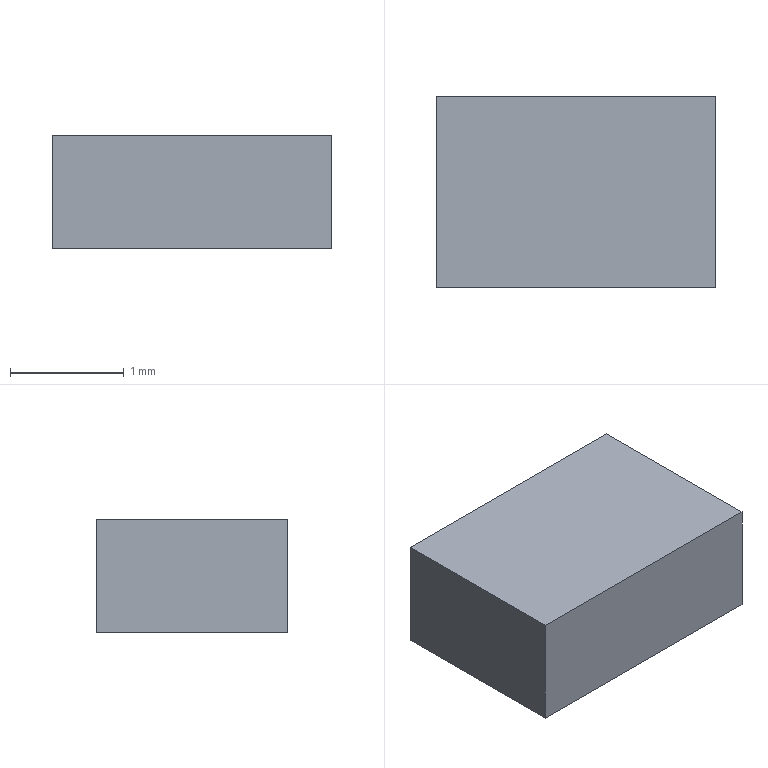Part | Creo | 1 solid | 6 faces | box 2.45 x 1.685 x 1 mm | volume 4.128 mm3 | plane 6
STEP:
#1=CARTESIAN_POINT('',(0.,0.,0.));
#2=DIRECTION('',(0.,0.,1.));
#3=DIRECTION('',(1.,0.,0.));
#4=AXIS2_PLACEMENT_3D('',#1,#2,#3);
#5=CARTESIAN_POINT('',(-1.3,-0.91,0.));
#6=VERTEX_POINT('',#5);
#7=CARTESIAN_POINT('',(1.15,-0.91,0.));
#8=VERTEX_POINT('',#7);
#9=CARTESIAN_POINT('',(-1.3,-0.91,0.));
#10=DIRECTION('',(1.,0.,0.));
#11=VECTOR('',#10,2.45);
#12=LINE('',#9,#11);
#13=EDGE_CURVE('',#6,#8,#12,.T.);
#14=ORIENTED_EDGE('',*,*,#13,.T.);
#15=CARTESIAN_POINT('',(1.15,0.775,0.));
#16=VERTEX_POINT('',#15);
#17=CARTESIAN_POINT('',(1.15,-0.91,0.));
#18=DIRECTION('',(0.,1.,0.));
#19=VECTOR('',#18,1.685);
#20=LINE('',#17,#19);
#21=EDGE_CURVE('',#8,#16,#20,.T.);
#22=ORIENTED_EDGE('',*,*,#21,.T.);
#23=CARTESIAN_POINT('',(-1.3,0.775,0.));
#24=VERTEX_POINT('',#23);
#25=CARTESIAN_POINT('',(1.15,0.775,0.));
#26=DIRECTION('',(-1.,0.,0.));
#27=VECTOR('',#26,2.45);
#28=LINE('',#25,#27);
#29=EDGE_CURVE('',#16,#24,#28,.T.);
#30=ORIENTED_EDGE('',*,*,#29,.T.);
#31=CARTESIAN_POINT('',(-1.3,0.775,0.));
#32=DIRECTION('',(0.,-1.,0.));
#33=VECTOR('',#32,1.685);
#34=LINE('',#31,#33);
#35=EDGE_CURVE('',#24,#6,#34,.T.);
#36=ORIENTED_EDGE('',*,*,#35,.T.);
#37=EDGE_LOOP('',(#14,#22,#30,#36));
#38=FACE_OUTER_BOUND('',#37,.F.);
#39=CARTESIAN_POINT('',(0.,0.,0.));
#40=DIRECTION('',(0.,0.,1.));
#41=DIRECTION('',(1.,0.,0.));
#42=AXIS2_PLACEMENT_3D('',#39,#40,#41);
#43=PLANE('',#42);
#44=ADVANCED_FACE('',(#38),#43,.F.);
#45=ORIENTED_EDGE('',*,*,#13,.F.);
#46=CARTESIAN_POINT('',(-1.3,-0.91,1.));
#47=VERTEX_POINT('',#46);
#48=CARTESIAN_POINT('',(-1.3,-0.91,0.));
#49=DIRECTION('',(0.,0.,1.));
#50=VECTOR('',#49,1.);
#51=LINE('',#48,#50);
#52=EDGE_CURVE('',#6,#47,#51,.T.);
#53=ORIENTED_EDGE('',*,*,#52,.T.);
#54=CARTESIAN_POINT('',(1.15,-0.91,1.));
#55=VERTEX_POINT('',#54);
#56=CARTESIAN_POINT('',(-1.3,-0.91,1.));
#57=DIRECTION('',(1.,0.,0.));
#58=VECTOR('',#57,2.45);
#59=LINE('',#56,#58);
#60=EDGE_CURVE('',#47,#55,#59,.T.);
#61=ORIENTED_EDGE('',*,*,#60,.T.);
#62=CARTESIAN_POINT('',(1.15,-0.91,0.));
#63=DIRECTION('',(0.,0.,1.));
#64=VECTOR('',#63,1.);
#65=LINE('',#62,#64);
#66=EDGE_CURVE('',#8,#55,#65,.T.);
#67=ORIENTED_EDGE('',*,*,#66,.F.);
#68=EDGE_LOOP('',(#45,#53,#61,#67));
#69=FACE_OUTER_BOUND('',#68,.F.);
#70=CARTESIAN_POINT('',(-1.3,-0.91,0.));
#71=DIRECTION('',(0.,-1.,0.));
#72=DIRECTION('',(1.,0.,0.));
#73=AXIS2_PLACEMENT_3D('',#70,#71,#72);
#74=PLANE('',#73);
#75=ADVANCED_FACE('',(#69),#74,.T.);
#76=ORIENTED_EDGE('',*,*,#35,.F.);
#77=CARTESIAN_POINT('',(-1.3,0.775,1.));
#78=VERTEX_POINT('',#77);
#79=CARTESIAN_POINT('',(-1.3,0.775,0.));
#80=DIRECTION('',(0.,0.,1.));
#81=VECTOR('',#80,1.);
#82=LINE('',#79,#81);
#83=EDGE_CURVE('',#24,#78,#82,.T.);
#84=ORIENTED_EDGE('',*,*,#83,.T.);
#85=CARTESIAN_POINT('',(-1.3,0.775,1.));
#86=DIRECTION('',(0.,-1.,0.));
#87=VECTOR('',#86,1.685);
#88=LINE('',#85,#87);
#89=EDGE_CURVE('',#78,#47,#88,.T.);
#90=ORIENTED_EDGE('',*,*,#89,.T.);
#91=ORIENTED_EDGE('',*,*,#52,.F.);
#92=EDGE_LOOP('',(#76,#84,#90,#91));
#93=FACE_OUTER_BOUND('',#92,.F.);
#94=CARTESIAN_POINT('',(-1.3,0.775,0.));
#95=DIRECTION('',(-1.,0.,0.));
#96=DIRECTION('',(0.,-1.,0.));
#97=AXIS2_PLACEMENT_3D('',#94,#95,#96);
#98=PLANE('',#97);
#99=ADVANCED_FACE('',(#93),#98,.T.);
#100=ORIENTED_EDGE('',*,*,#29,.F.);
#101=CARTESIAN_POINT('',(1.15,0.775,1.));
#102=VERTEX_POINT('',#101);
#103=CARTESIAN_POINT('',(1.15,0.775,0.));
#104=DIRECTION('',(0.,0.,1.));
#105=VECTOR('',#104,1.);
#106=LINE('',#103,#105);
#107=EDGE_CURVE('',#16,#102,#106,.T.);
#108=ORIENTED_EDGE('',*,*,#107,.T.);
#109=CARTESIAN_POINT('',(1.15,0.775,1.));
#110=DIRECTION('',(-1.,0.,0.));
#111=VECTOR('',#110,2.45);
#112=LINE('',#109,#111);
#113=EDGE_CURVE('',#102,#78,#112,.T.);
#114=ORIENTED_EDGE('',*,*,#113,.T.);
#115=ORIENTED_EDGE('',*,*,#83,.F.);
#116=EDGE_LOOP('',(#100,#108,#114,#115));
#117=FACE_OUTER_BOUND('',#116,.F.);
#118=CARTESIAN_POINT('',(1.15,0.775,0.));
#119=DIRECTION('',(0.,1.,0.));
#120=DIRECTION('',(-1.,0.,0.));
#121=AXIS2_PLACEMENT_3D('',#118,#119,#120);
#122=PLANE('',#121);
#123=ADVANCED_FACE('',(#117),#122,.T.);
#124=ORIENTED_EDGE('',*,*,#21,.F.);
#125=ORIENTED_EDGE('',*,*,#66,.T.);
#126=CARTESIAN_POINT('',(1.15,-0.91,1.));
#127=DIRECTION('',(0.,1.,0.));
#128=VECTOR('',#127,1.685);
#129=LINE('',#126,#128);
#130=EDGE_CURVE('',#55,#102,#129,.T.);
#131=ORIENTED_EDGE('',*,*,#130,.T.);
#132=ORIENTED_EDGE('',*,*,#107,.F.);
#133=EDGE_LOOP('',(#124,#125,#131,#132));
#134=FACE_OUTER_BOUND('',#133,.F.);
#135=CARTESIAN_POINT('',(1.15,-0.91,0.));
#136=DIRECTION('',(1.,0.,0.));
#137=DIRECTION('',(0.,1.,0.));
#138=AXIS2_PLACEMENT_3D('',#135,#136,#137);
#139=PLANE('',#138);
#140=ADVANCED_FACE('',(#134),#139,.T.);
#141=ORIENTED_EDGE('',*,*,#60,.F.);
#142=ORIENTED_EDGE('',*,*,#89,.F.);
#143=ORIENTED_EDGE('',*,*,#113,.F.);
#144=ORIENTED_EDGE('',*,*,#130,.F.);
#145=EDGE_LOOP('',(#141,#142,#143,#144));
#146=FACE_OUTER_BOUND('',#145,.F.);
#147=CARTESIAN_POINT('',(0.,0.,1.));
#148=DIRECTION('',(0.,0.,1.));
#149=DIRECTION('',(1.,0.,0.));
#150=AXIS2_PLACEMENT_3D('',#147,#148,#149);
#151=PLANE('',#150);
#152=ADVANCED_FACE('',(#146),#151,.T.);
#153=CLOSED_SHELL('',(#44,#75,#99,#123,#140,#152));
#154=MANIFOLD_SOLID_BREP('',#153);
#155=(LENGTH_UNIT()NAMED_UNIT(*)SI_UNIT(.MILLI.,.METRE.));
#156=UNCERTAINTY_MEASURE_WITH_UNIT(LENGTH_MEASURE(0.0003137),#155,'','');
#157=(NAMED_UNIT(*)PLANE_ANGLE_UNIT()SI_UNIT($,.RADIAN.));
#158=PLANE_ANGLE_MEASURE_WITH_UNIT(PLANE_ANGLE_MEASURE(0.01745),#157);
#159=(CONVERSION_BASED_UNIT('DEGREE',#158)NAMED_UNIT(*)PLANE_ANGLE_UNIT());
#160=(NAMED_UNIT(*)SI_UNIT($,.STERADIAN.)SOLID_ANGLE_UNIT());
#161=(GEOMETRIC_REPRESENTATION_CONTEXT(3)GLOBAL_UNCERTAINTY_ASSIGNED_CONTEXT((#156))GLOBAL_UNIT_ASSIGNED_CONTEXT((#155,#159,#160))REPRESENTATION_CONTEXT('',''));
#162=ADVANCED_BREP_SHAPE_REPRESENTATION('',(#4,#154),#161);